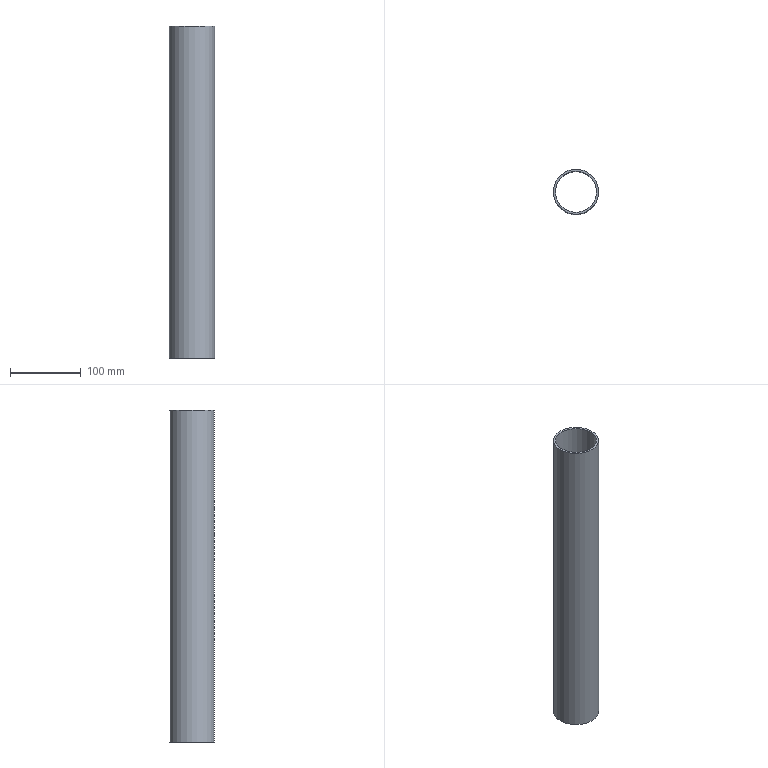Part | STEP file | JBJ-P-1000-07 | 1 solid | 4 faces | box 64 x 64 x 470 mm | volume 270208 mm3 | plane 2 | cylinder 2 | commonest cylinder face diameters 58 x1 64 x1
STEP:
#1=CARTESIAN_POINT('',(32.,0.,470.));
#2=VERTEX_POINT('',#1);
#3=CARTESIAN_POINT('',(0.,0.,470.));
#4=DIRECTION('',(0.,0.,1.));
#5=DIRECTION('',(1.,0.,0.));
#6=AXIS2_PLACEMENT_3D('',#3,#4,#5);
#7=CIRCLE('',#6,32.);
#8=EDGE_CURVE('',#2,#2,#7,.T.);
#9=ORIENTED_EDGE('',*,*,#8,.T.);
#10=EDGE_LOOP('',(#9));
#11=FACE_OUTER_BOUND('',#10,.T.);
#12=CARTESIAN_POINT('',(29.,0.,470.));
#13=VERTEX_POINT('',#12);
#14=CARTESIAN_POINT('',(0.,0.,470.));
#15=DIRECTION('',(0.,0.,1.));
#16=DIRECTION('',(1.,0.,0.));
#17=AXIS2_PLACEMENT_3D('',#14,#15,#16);
#18=CIRCLE('',#17,29.);
#19=EDGE_CURVE('',#13,#13,#18,.T.);
#20=ORIENTED_EDGE('',*,*,#19,.F.);
#21=EDGE_LOOP('',(#20));
#22=FACE_BOUND('',#21,.T.);
#23=CARTESIAN_POINT('',(0.,0.,470.));
#24=DIRECTION('',(0.,0.,1.));
#25=DIRECTION('',(1.,0.,0.));
#26=AXIS2_PLACEMENT_3D('',#23,#24,#25);
#27=PLANE('',#26);
#28=ADVANCED_FACE('',(#11,#22),#27,.T.);
#29=CARTESIAN_POINT('',(32.,0.,0.));
#30=VERTEX_POINT('',#29);
#31=CARTESIAN_POINT('',(0.,0.,0.));
#32=DIRECTION('',(0.,0.,1.));
#33=DIRECTION('',(1.,0.,0.));
#34=AXIS2_PLACEMENT_3D('',#31,#32,#33);
#35=CIRCLE('',#34,32.);
#36=EDGE_CURVE('',#30,#30,#35,.T.);
#37=ORIENTED_EDGE('',*,*,#36,.F.);
#38=EDGE_LOOP('',(#37));
#39=FACE_OUTER_BOUND('',#38,.T.);
#40=CARTESIAN_POINT('',(29.,0.,0.));
#41=VERTEX_POINT('',#40);
#42=CARTESIAN_POINT('',(0.,0.,0.));
#43=DIRECTION('',(0.,0.,1.));
#44=DIRECTION('',(1.,0.,0.));
#45=AXIS2_PLACEMENT_3D('',#42,#43,#44);
#46=CIRCLE('',#45,29.);
#47=EDGE_CURVE('',#41,#41,#46,.T.);
#48=ORIENTED_EDGE('',*,*,#47,.T.);
#49=EDGE_LOOP('',(#48));
#50=FACE_BOUND('',#49,.T.);
#51=CARTESIAN_POINT('',(0.,0.,0.));
#52=DIRECTION('',(0.,0.,1.));
#53=DIRECTION('',(1.,0.,0.));
#54=AXIS2_PLACEMENT_3D('',#51,#52,#53);
#55=PLANE('',#54);
#56=ADVANCED_FACE('',(#39,#50),#55,.F.);
#57=ORIENTED_EDGE('',*,*,#8,.F.);
#58=EDGE_LOOP('',(#57));
#59=FACE_OUTER_BOUND('',#58,.T.);
#60=ORIENTED_EDGE('',*,*,#36,.T.);
#61=EDGE_LOOP('',(#60));
#62=FACE_OUTER_BOUND('',#61,.T.);
#63=CARTESIAN_POINT('',(0.,0.,470.));
#64=DIRECTION('',(0.,0.,-1.));
#65=DIRECTION('',(-1.,0.,0.));
#66=AXIS2_PLACEMENT_3D('',#63,#64,#65);
#67=CYLINDRICAL_SURFACE('',#66,32.);
#68=ADVANCED_FACE('',(#59,#62),#67,.T.);
#69=ORIENTED_EDGE('',*,*,#19,.T.);
#70=EDGE_LOOP('',(#69));
#71=FACE_OUTER_BOUND('',#70,.T.);
#72=ORIENTED_EDGE('',*,*,#47,.F.);
#73=EDGE_LOOP('',(#72));
#74=FACE_OUTER_BOUND('',#73,.T.);
#75=CARTESIAN_POINT('',(0.,0.,470.));
#76=DIRECTION('',(0.,0.,-1.));
#77=DIRECTION('',(-1.,0.,0.));
#78=AXIS2_PLACEMENT_3D('',#75,#76,#77);
#79=CYLINDRICAL_SURFACE('',#78,29.);
#80=ADVANCED_FACE('',(#71,#74),#79,.F.);
#81=CLOSED_SHELL('',(#28,#56,#68,#80));
#82=MANIFOLD_SOLID_BREP('',#81);
#83=CARTESIAN_POINT('',(0.,0.,0.));
#84=DIRECTION('',(0.,0.,1.));
#85=DIRECTION('',(1.,0.,0.));
#86=AXIS2_PLACEMENT_3D('',#83,#84,#85);
#87=(LENGTH_UNIT()NAMED_UNIT(*)SI_UNIT(.MILLI.,.METRE.));
#88=UNCERTAINTY_MEASURE_WITH_UNIT(LENGTH_MEASURE(0.00001),#87,'','');
#89=(NAMED_UNIT(*)PLANE_ANGLE_UNIT()SI_UNIT($,.RADIAN.));
#90=(NAMED_UNIT(*)SI_UNIT($,.STERADIAN.)SOLID_ANGLE_UNIT());
#91=(GEOMETRIC_REPRESENTATION_CONTEXT(3)GLOBAL_UNCERTAINTY_ASSIGNED_CONTEXT((#88))GLOBAL_UNIT_ASSIGNED_CONTEXT((#87,#89,#90))REPRESENTATION_CONTEXT('',''));
#92=ADVANCED_BREP_SHAPE_REPRESENTATION('',(#82,#86),#91);